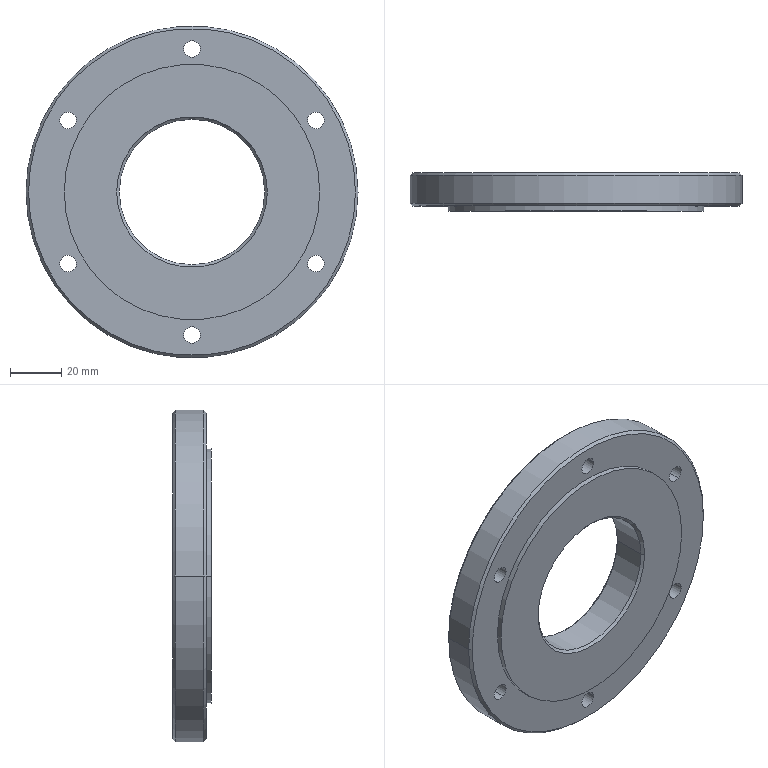Part | Creo | features CUT 7, CURVE 3, DATUM PLANE 3, CHAMFER 1, COORDINATE SYSTEM 1, PATTERN 1, PROTRUSION 1 | 1 solid | 47 faces | box 130 x 15 x 130 mm | volume 144210 mm3 | cylinder 30 | plane 9 | cone 8 | commonest cylinder face diameters 6.5 x12 11 x12 57 x2 100 x2 130 x2
STEP:
#1=CARTESIAN_POINT('',(0.,0.,0.));
#2=DIRECTION('',(0.,0.,1.));
#3=DIRECTION('',(1.,0.,0.));
#4=AXIS2_PLACEMENT_3D('',#1,#2,#3);
#5=CARTESIAN_POINT('',(50.,0.,0.));
#6=VERTEX_POINT('',#5);
#7=CARTESIAN_POINT('',(-50.,0.,0.));
#8=VERTEX_POINT('',#7);
#9=CARTESIAN_POINT('',(0.,0.,0.));
#10=DIRECTION('',(0.,-1.,0.));
#11=DIRECTION('',(1.,0.,0.));
#12=AXIS2_PLACEMENT_3D('',#9,#10,#11);
#13=CIRCLE('',#12,50.);
#14=EDGE_CURVE('',#6,#8,#13,.T.);
#15=ORIENTED_EDGE('',*,*,#14,.F.);
#16=CARTESIAN_POINT('',(0.,0.,0.));
#17=DIRECTION('',(0.,1.,0.));
#18=DIRECTION('',(1.,0.,0.));
#19=AXIS2_PLACEMENT_3D('',#16,#17,#18);
#20=CIRCLE('',#19,50.);
#21=EDGE_CURVE('',#6,#8,#20,.T.);
#22=ORIENTED_EDGE('',*,*,#21,.T.);
#23=EDGE_LOOP('',(#15,#22));
#24=FACE_OUTER_BOUND('',#23,.F.);
#25=CARTESIAN_POINT('',(-29.5,0.,0.));
#26=VERTEX_POINT('',#25);
#27=CARTESIAN_POINT('',(29.5,0.,0.));
#28=VERTEX_POINT('',#27);
#29=CARTESIAN_POINT('',(0.,0.,0.));
#30=DIRECTION('',(0.,1.,0.));
#31=DIRECTION('',(-1.,0.,0.));
#32=AXIS2_PLACEMENT_3D('',#29,#30,#31);
#33=CIRCLE('',#32,29.5);
#34=EDGE_CURVE('',#26,#28,#33,.T.);
#35=ORIENTED_EDGE('',*,*,#34,.F.);
#36=CARTESIAN_POINT('',(0.,0.,0.));
#37=DIRECTION('',(0.,1.,0.));
#38=DIRECTION('',(1.,0.,0.));
#39=AXIS2_PLACEMENT_3D('',#36,#37,#38);
#40=CIRCLE('',#39,29.5);
#41=EDGE_CURVE('',#28,#26,#40,.T.);
#42=ORIENTED_EDGE('',*,*,#41,.F.);
#43=EDGE_LOOP('',(#35,#42));
#44=FACE_BOUND('',#43,.F.);
#45=CARTESIAN_POINT('',(0.,0.,0.));
#46=DIRECTION('',(0.,1.,0.));
#47=DIRECTION('',(1.,0.,0.));
#48=AXIS2_PLACEMENT_3D('',#45,#46,#47);
#49=PLANE('',#48);
#50=ADVANCED_FACE('',(#24,#44),#49,.F.);
#51=CARTESIAN_POINT('',(50.,2.,0.));
#52=VERTEX_POINT('',#51);
#53=CARTESIAN_POINT('',(50.,0.,0.));
#54=DIRECTION('',(0.,1.,0.));
#55=VECTOR('',#54,2.);
#56=LINE('',#53,#55);
#57=EDGE_CURVE('',#6,#52,#56,.T.);
#58=ORIENTED_EDGE('',*,*,#57,.F.);
#59=ORIENTED_EDGE('',*,*,#14,.T.);
#60=CARTESIAN_POINT('',(-50.,2.,0.));
#61=VERTEX_POINT('',#60);
#62=CARTESIAN_POINT('',(-50.,0.,0.));
#63=DIRECTION('',(0.,1.,0.));
#64=VECTOR('',#63,2.);
#65=LINE('',#62,#64);
#66=EDGE_CURVE('',#8,#61,#65,.T.);
#67=ORIENTED_EDGE('',*,*,#66,.T.);
#68=CARTESIAN_POINT('',(0.,2.,0.));
#69=DIRECTION('',(0.,-1.,0.));
#70=DIRECTION('',(1.,0.,0.));
#71=AXIS2_PLACEMENT_3D('',#68,#69,#70);
#72=CIRCLE('',#71,50.);
#73=EDGE_CURVE('',#52,#61,#72,.T.);
#74=ORIENTED_EDGE('',*,*,#73,.F.);
#75=EDGE_LOOP('',(#58,#59,#67,#74));
#76=FACE_OUTER_BOUND('',#75,.F.);
#77=CARTESIAN_POINT('',(0.,0.,0.));
#78=DIRECTION('',(0.,1.,0.));
#79=DIRECTION('',(1.,0.,0.));
#80=AXIS2_PLACEMENT_3D('',#77,#78,#79);
#81=CYLINDRICAL_SURFACE('',#80,50.);
#82=ADVANCED_FACE('',(#76),#81,.T.);
#83=ORIENTED_EDGE('',*,*,#57,.T.);
#84=CARTESIAN_POINT('',(0.,2.,0.));
#85=DIRECTION('',(0.,1.,0.));
#86=DIRECTION('',(1.,0.,0.));
#87=AXIS2_PLACEMENT_3D('',#84,#85,#86);
#88=CIRCLE('',#87,50.);
#89=EDGE_CURVE('',#52,#61,#88,.T.);
#90=ORIENTED_EDGE('',*,*,#89,.T.);
#91=ORIENTED_EDGE('',*,*,#66,.F.);
#92=ORIENTED_EDGE('',*,*,#21,.F.);
#93=EDGE_LOOP('',(#83,#90,#91,#92));
#94=FACE_OUTER_BOUND('',#93,.F.);
#95=CARTESIAN_POINT('',(0.,0.,0.));
#96=DIRECTION('',(0.,1.,0.));
#97=DIRECTION('',(1.,0.,0.));
#98=AXIS2_PLACEMENT_3D('',#95,#96,#97);
#99=CYLINDRICAL_SURFACE('',#98,50.);
#100=ADVANCED_FACE('',(#94),#99,.T.);
#101=CARTESIAN_POINT('',(-64.,2.,0.));
#102=VERTEX_POINT('',#101);
#103=CARTESIAN_POINT('',(64.,2.,0.));
#104=VERTEX_POINT('',#103);
#105=CARTESIAN_POINT('',(0.,2.,0.));
#106=DIRECTION('',(0.,1.,0.));
#107=DIRECTION('',(-1.,0.,0.));
#108=AXIS2_PLACEMENT_3D('',#105,#106,#107);
#109=CIRCLE('',#108,64.);
#110=EDGE_CURVE('',#102,#104,#109,.T.);
#111=ORIENTED_EDGE('',*,*,#110,.T.);
#112=CARTESIAN_POINT('',(0.,2.,0.));
#113=DIRECTION('',(0.,1.,0.));
#114=DIRECTION('',(1.,0.,0.));
#115=AXIS2_PLACEMENT_3D('',#112,#113,#114);
#116=CIRCLE('',#115,64.);
#117=EDGE_CURVE('',#104,#102,#116,.T.);
#118=ORIENTED_EDGE('',*,*,#117,.T.);
#119=EDGE_LOOP('',(#111,#118));
#120=FACE_OUTER_BOUND('',#119,.F.);
#121=CARTESIAN_POINT('',(3.25,2.,-56.));
#122=VERTEX_POINT('',#121);
#123=CARTESIAN_POINT('',(-3.25,2.,-56.));
#124=VERTEX_POINT('',#123);
#125=CARTESIAN_POINT('',(0.,2.,-56.));
#126=DIRECTION('',(0.,1.,0.));
#127=DIRECTION('',(1.,0.,0.));
#128=AXIS2_PLACEMENT_3D('',#125,#126,#127);
#129=CIRCLE('',#128,3.25);
#130=EDGE_CURVE('',#122,#124,#129,.T.);
#131=ORIENTED_EDGE('',*,*,#130,.F.);
#132=CARTESIAN_POINT('',(0.,2.,-56.));
#133=DIRECTION('',(0.,1.,0.));
#134=DIRECTION('',(-1.,0.,0.));
#135=AXIS2_PLACEMENT_3D('',#132,#133,#134);
#136=CIRCLE('',#135,3.25);
#137=EDGE_CURVE('',#124,#122,#136,.T.);
#138=ORIENTED_EDGE('',*,*,#137,.F.);
#139=EDGE_LOOP('',(#131,#138));
#140=FACE_BOUND('',#139,.F.);
#141=CARTESIAN_POINT('',(-46.872,2.,-30.815));
#142=VERTEX_POINT('',#141);
#143=CARTESIAN_POINT('',(-50.122,2.,-25.185));
#144=VERTEX_POINT('',#143);
#145=CARTESIAN_POINT('',(-48.497,2.,-28.));
#146=DIRECTION('',(0.,1.,0.));
#147=DIRECTION('',(0.5,0.,-0.866));
#148=AXIS2_PLACEMENT_3D('',#145,#146,#147);
#149=CIRCLE('',#148,3.25);
#150=EDGE_CURVE('',#142,#144,#149,.T.);
#151=ORIENTED_EDGE('',*,*,#150,.F.);
#152=CARTESIAN_POINT('',(-48.497,2.,-28.));
#153=DIRECTION('',(0.,1.,0.));
#154=DIRECTION('',(-0.5,0.,0.866));
#155=AXIS2_PLACEMENT_3D('',#152,#153,#154);
#156=CIRCLE('',#155,3.25);
#157=EDGE_CURVE('',#144,#142,#156,.T.);
#158=ORIENTED_EDGE('',*,*,#157,.F.);
#159=EDGE_LOOP('',(#151,#158));
#160=FACE_BOUND('',#159,.F.);
#161=CARTESIAN_POINT('',(-50.122,2.,25.185));
#162=VERTEX_POINT('',#161);
#163=CARTESIAN_POINT('',(-46.872,2.,30.815));
#164=VERTEX_POINT('',#163);
#165=CARTESIAN_POINT('',(-48.497,2.,28.));
#166=DIRECTION('',(0.,1.,0.));
#167=DIRECTION('',(-0.5,0.,-0.866));
#168=AXIS2_PLACEMENT_3D('',#165,#166,#167);
#169=CIRCLE('',#168,3.25);
#170=EDGE_CURVE('',#162,#164,#169,.T.);
#171=ORIENTED_EDGE('',*,*,#170,.F.);
#172=CARTESIAN_POINT('',(-48.497,2.,28.));
#173=DIRECTION('',(0.,1.,0.));
#174=DIRECTION('',(0.5,0.,0.866));
#175=AXIS2_PLACEMENT_3D('',#172,#173,#174);
#176=CIRCLE('',#175,3.25);
#177=EDGE_CURVE('',#164,#162,#176,.T.);
#178=ORIENTED_EDGE('',*,*,#177,.F.);
#179=EDGE_LOOP('',(#171,#178));
#180=FACE_BOUND('',#179,.F.);
#181=CARTESIAN_POINT('',(-3.25,2.,56.));
#182=VERTEX_POINT('',#181);
#183=CARTESIAN_POINT('',(3.25,2.,56.));
#184=VERTEX_POINT('',#183);
#185=CARTESIAN_POINT('',(0.,2.,56.));
#186=DIRECTION('',(0.,1.,0.));
#187=DIRECTION('',(-1.,0.,0.));
#188=AXIS2_PLACEMENT_3D('',#185,#186,#187);
#189=CIRCLE('',#188,3.25);
#190=EDGE_CURVE('',#182,#184,#189,.T.);
#191=ORIENTED_EDGE('',*,*,#190,.F.);
#192=CARTESIAN_POINT('',(0.,2.,56.));
#193=DIRECTION('',(0.,1.,0.));
#194=DIRECTION('',(1.,0.,0.));
#195=AXIS2_PLACEMENT_3D('',#192,#193,#194);
#196=CIRCLE('',#195,3.25);
#197=EDGE_CURVE('',#184,#182,#196,.T.);
#198=ORIENTED_EDGE('',*,*,#197,.F.);
#199=EDGE_LOOP('',(#191,#198));
#200=FACE_BOUND('',#199,.F.);
#201=CARTESIAN_POINT('',(46.872,2.,30.815));
#202=VERTEX_POINT('',#201);
#203=CARTESIAN_POINT('',(50.122,2.,25.185));
#204=VERTEX_POINT('',#203);
#205=CARTESIAN_POINT('',(48.497,2.,28.));
#206=DIRECTION('',(0.,1.,0.));
#207=DIRECTION('',(-0.5,0.,0.866));
#208=AXIS2_PLACEMENT_3D('',#205,#206,#207);
#209=CIRCLE('',#208,3.25);
#210=EDGE_CURVE('',#202,#204,#209,.T.);
#211=ORIENTED_EDGE('',*,*,#210,.F.);
#212=CARTESIAN_POINT('',(48.497,2.,28.));
#213=DIRECTION('',(0.,1.,0.));
#214=DIRECTION('',(0.5,0.,-0.866));
#215=AXIS2_PLACEMENT_3D('',#212,#213,#214);
#216=CIRCLE('',#215,3.25);
#217=EDGE_CURVE('',#204,#202,#216,.T.);
#218=ORIENTED_EDGE('',*,*,#217,.F.);
#219=EDGE_LOOP('',(#211,#218));
#220=FACE_BOUND('',#219,.F.);
#221=CARTESIAN_POINT('',(50.122,2.,-25.185));
#222=VERTEX_POINT('',#221);
#223=CARTESIAN_POINT('',(46.872,2.,-30.815));
#224=VERTEX_POINT('',#223);
#225=CARTESIAN_POINT('',(48.497,2.,-28.));
#226=DIRECTION('',(0.,1.,0.));
#227=DIRECTION('',(0.5,0.,0.866));
#228=AXIS2_PLACEMENT_3D('',#225,#226,#227);
#229=CIRCLE('',#228,3.25);
#230=EDGE_CURVE('',#222,#224,#229,.T.);
#231=ORIENTED_EDGE('',*,*,#230,.F.);
#232=CARTESIAN_POINT('',(48.497,2.,-28.));
#233=DIRECTION('',(0.,1.,0.));
#234=DIRECTION('',(-0.5,0.,-0.866));
#235=AXIS2_PLACEMENT_3D('',#232,#233,#234);
#236=CIRCLE('',#235,3.25);
#237=EDGE_CURVE('',#224,#222,#236,.T.);
#238=ORIENTED_EDGE('',*,*,#237,.F.);
#239=EDGE_LOOP('',(#231,#238));
#240=FACE_BOUND('',#239,.F.);
#241=ORIENTED_EDGE('',*,*,#89,.F.);
#242=ORIENTED_EDGE('',*,*,#73,.T.);
#243=EDGE_LOOP('',(#241,#242));
#244=FACE_BOUND('',#243,.F.);
#245=CARTESIAN_POINT('',(0.,2.,0.));
#246=DIRECTION('',(0.,1.,0.));
#247=DIRECTION('',(1.,0.,0.));
#248=AXIS2_PLACEMENT_3D('',#245,#246,#247);
#249=PLANE('',#248);
#250=ADVANCED_FACE('',(#120,#140,#160,#180,#200,#220,#240,#244),#249,.F.);
#251=CARTESIAN_POINT('',(3.25,8.,-56.));
#252=VERTEX_POINT('',#251);
#253=CARTESIAN_POINT('',(-3.25,8.,-56.));
#254=VERTEX_POINT('',#253);
#255=CARTESIAN_POINT('',(0.,8.,-56.));
#256=DIRECTION('',(0.,1.,0.));
#257=DIRECTION('',(1.,0.,0.));
#258=AXIS2_PLACEMENT_3D('',#255,#256,#257);
#259=CIRCLE('',#258,3.25);
#260=EDGE_CURVE('',#252,#254,#259,.T.);
#261=ORIENTED_EDGE('',*,*,#260,.F.);
#262=CARTESIAN_POINT('',(3.25,8.,-56.));
#263=DIRECTION('',(0.,-1.,0.));
#264=VECTOR('',#263,6.);
#265=LINE('',#262,#264);
#266=EDGE_CURVE('',#252,#122,#265,.T.);
#267=ORIENTED_EDGE('',*,*,#266,.T.);
#268=ORIENTED_EDGE('',*,*,#130,.T.);
#269=CARTESIAN_POINT('',(-3.25,8.,-56.));
#270=DIRECTION('',(0.,-1.,0.));
#271=VECTOR('',#270,6.);
#272=LINE('',#269,#271);
#273=EDGE_CURVE('',#254,#124,#272,.T.);
#274=ORIENTED_EDGE('',*,*,#273,.F.);
#275=EDGE_LOOP('',(#261,#267,#268,#274));
#276=FACE_OUTER_BOUND('',#275,.F.);
#277=CARTESIAN_POINT('',(0.,15.,-56.));
#278=DIRECTION('',(0.,1.,0.));
#279=DIRECTION('',(1.,0.,0.));
#280=AXIS2_PLACEMENT_3D('',#277,#278,#279);
#281=CYLINDRICAL_SURFACE('',#280,3.25);
#282=ADVANCED_FACE('',(#276),#281,.F.);
#283=CARTESIAN_POINT('',(5.5,8.,-56.));
#284=VERTEX_POINT('',#283);
#285=CARTESIAN_POINT('',(-5.5,8.,-56.));
#286=VERTEX_POINT('',#285);
#287=CARTESIAN_POINT('',(0.,8.,-56.));
#288=DIRECTION('',(0.,1.,0.));
#289=DIRECTION('',(1.,0.,0.));
#290=AXIS2_PLACEMENT_3D('',#287,#288,#289);
#291=CIRCLE('',#290,5.5);
#292=EDGE_CURVE('',#284,#286,#291,.T.);
#293=ORIENTED_EDGE('',*,*,#292,.F.);
#294=CARTESIAN_POINT('',(0.,8.,-56.));
#295=DIRECTION('',(0.,1.,0.));
#296=DIRECTION('',(-1.,0.,0.));
#297=AXIS2_PLACEMENT_3D('',#294,#295,#296);
#298=CIRCLE('',#297,5.5);
#299=EDGE_CURVE('',#286,#284,#298,.T.);
#300=ORIENTED_EDGE('',*,*,#299,.F.);
#301=EDGE_LOOP('',(#293,#300));
#302=FACE_OUTER_BOUND('',#301,.F.);
#303=ORIENTED_EDGE('',*,*,#260,.T.);
#304=CARTESIAN_POINT('',(0.,8.,-56.));
#305=DIRECTION('',(0.,1.,0.));
#306=DIRECTION('',(-1.,0.,0.));
#307=AXIS2_PLACEMENT_3D('',#304,#305,#306);
#308=CIRCLE('',#307,3.25);
#309=EDGE_CURVE('',#254,#252,#308,.T.);
#310=ORIENTED_EDGE('',*,*,#309,.T.);
#311=EDGE_LOOP('',(#303,#310));
#312=FACE_BOUND('',#311,.F.);
#313=CARTESIAN_POINT('',(0.,8.,0.));
#314=DIRECTION('',(0.,1.,0.));
#315=DIRECTION('',(1.,0.,0.));
#316=AXIS2_PLACEMENT_3D('',#313,#314,#315);
#317=PLANE('',#316);
#318=ADVANCED_FACE('',(#302,#312),#317,.T.);
#319=CARTESIAN_POINT('',(53.997,8.,-28.));
#320=VERTEX_POINT('',#319);
#321=CARTESIAN_POINT('',(42.997,8.,-28.));
#322=VERTEX_POINT('',#321);
#323=CARTESIAN_POINT('',(48.497,8.,-28.));
#324=DIRECTION('',(0.,1.,0.));
#325=DIRECTION('',(1.,0.,0.));
#326=AXIS2_PLACEMENT_3D('',#323,#324,#325);
#327=CIRCLE('',#326,5.5);
#328=EDGE_CURVE('',#320,#322,#327,.T.);
#329=ORIENTED_EDGE('',*,*,#328,.F.);
#330=CARTESIAN_POINT('',(48.497,8.,-28.));
#331=DIRECTION('',(0.,1.,0.));
#332=DIRECTION('',(-1.,0.,0.));
#333=AXIS2_PLACEMENT_3D('',#330,#331,#332);
#334=CIRCLE('',#333,5.5);
#335=EDGE_CURVE('',#322,#320,#334,.T.);
#336=ORIENTED_EDGE('',*,*,#335,.F.);
#337=EDGE_LOOP('',(#329,#336));
#338=FACE_OUTER_BOUND('',#337,.F.);
#339=CARTESIAN_POINT('',(50.122,8.,-25.185));
#340=VERTEX_POINT('',#339);
#341=CARTESIAN_POINT('',(46.872,8.,-30.815));
#342=VERTEX_POINT('',#341);
#343=CARTESIAN_POINT('',(48.497,8.,-28.));
#344=DIRECTION('',(0.,1.,0.));
#345=DIRECTION('',(0.5,0.,0.866));
#346=AXIS2_PLACEMENT_3D('',#343,#344,#345);
#347=CIRCLE('',#346,3.25);
#348=EDGE_CURVE('',#340,#342,#347,.T.);
#349=ORIENTED_EDGE('',*,*,#348,.T.);
#350=CARTESIAN_POINT('',(48.497,8.,-28.));
#351=DIRECTION('',(0.,1.,0.));
#352=DIRECTION('',(-0.5,0.,-0.866));
#353=AXIS2_PLACEMENT_3D('',#350,#351,#352);
#354=CIRCLE('',#353,3.25);
#355=EDGE_CURVE('',#342,#340,#354,.T.);
#356=ORIENTED_EDGE('',*,*,#355,.T.);
#357=EDGE_LOOP('',(#349,#356));
#358=FACE_BOUND('',#357,.F.);
#359=CARTESIAN_POINT('',(0.,8.,0.));
#360=DIRECTION('',(0.,1.,0.));
#361=DIRECTION('',(1.,0.,0.));
#362=AXIS2_PLACEMENT_3D('',#359,#360,#361);
#363=PLANE('',#362);
#364=ADVANCED_FACE('',(#338,#358),#363,.T.);
#365=CARTESIAN_POINT('',(53.997,8.,28.));
#366=VERTEX_POINT('',#365);
#367=CARTESIAN_POINT('',(42.997,8.,28.));
#368=VERTEX_POINT('',#367);
#369=CARTESIAN_POINT('',(48.497,8.,28.));
#370=DIRECTION('',(0.,1.,0.));
#371=DIRECTION('',(1.,0.,0.));
#372=AXIS2_PLACEMENT_3D('',#369,#370,#371);
#373=CIRCLE('',#372,5.5);
#374=EDGE_CURVE('',#366,#368,#373,.T.);
#375=ORIENTED_EDGE('',*,*,#374,.F.);
#376=CARTESIAN_POINT('',(48.497,8.,28.));
#377=DIRECTION('',(0.,1.,0.));
#378=DIRECTION('',(-1.,0.,0.));
#379=AXIS2_PLACEMENT_3D('',#376,#377,#378);
#380=CIRCLE('',#379,5.5);
#381=EDGE_CURVE('',#368,#366,#380,.T.);
#382=ORIENTED_EDGE('',*,*,#381,.F.);
#383=EDGE_LOOP('',(#375,#382));
#384=FACE_OUTER_BOUND('',#383,.F.);
#385=CARTESIAN_POINT('',(46.872,8.,30.815));
#386=VERTEX_POINT('',#385);
#387=CARTESIAN_POINT('',(50.122,8.,25.185));
#388=VERTEX_POINT('',#387);
#389=CARTESIAN_POINT('',(48.497,8.,28.));
#390=DIRECTION('',(0.,1.,0.));
#391=DIRECTION('',(-0.5,0.,0.866));
#392=AXIS2_PLACEMENT_3D('',#389,#390,#391);
#393=CIRCLE('',#392,3.25);
#394=EDGE_CURVE('',#386,#388,#393,.T.);
#395=ORIENTED_EDGE('',*,*,#394,.T.);
#396=CARTESIAN_POINT('',(48.497,8.,28.));
#397=DIRECTION('',(0.,1.,0.));
#398=DIRECTION('',(0.5,0.,-0.866));
#399=AXIS2_PLACEMENT_3D('',#396,#397,#398);
#400=CIRCLE('',#399,3.25);
#401=EDGE_CURVE('',#388,#386,#400,.T.);
#402=ORIENTED_EDGE('',*,*,#401,.T.);
#403=EDGE_LOOP('',(#395,#402));
#404=FACE_BOUND('',#403,.F.);
#405=CARTESIAN_POINT('',(0.,8.,0.));
#406=DIRECTION('',(0.,1.,0.));
#407=DIRECTION('',(1.,0.,0.));
#408=AXIS2_PLACEMENT_3D('',#405,#406,#407);
#409=PLANE('',#408);
#410=ADVANCED_FACE('',(#384,#404),#409,.T.);
#411=CARTESIAN_POINT('',(5.5,8.,56.));
#412=VERTEX_POINT('',#411);
#413=CARTESIAN_POINT('',(-5.5,8.,56.));
#414=VERTEX_POINT('',#413);
#415=CARTESIAN_POINT('',(0.,8.,56.));
#416=DIRECTION('',(0.,1.,0.));
#417=DIRECTION('',(1.,0.,0.));
#418=AXIS2_PLACEMENT_3D('',#415,#416,#417);
#419=CIRCLE('',#418,5.5);
#420=EDGE_CURVE('',#412,#414,#419,.T.);
#421=ORIENTED_EDGE('',*,*,#420,.F.);
#422=CARTESIAN_POINT('',(0.,8.,56.));
#423=DIRECTION('',(0.,1.,0.));
#424=DIRECTION('',(-1.,0.,0.));
#425=AXIS2_PLACEMENT_3D('',#422,#423,#424);
#426=CIRCLE('',#425,5.5);
#427=EDGE_CURVE('',#414,#412,#426,.T.);
#428=ORIENTED_EDGE('',*,*,#427,.F.);
#429=EDGE_LOOP('',(#421,#428));
#430=FACE_OUTER_BOUND('',#429,.F.);
#431=CARTESIAN_POINT('',(-3.25,8.,56.));
#432=VERTEX_POINT('',#431);
#433=CARTESIAN_POINT('',(3.25,8.,56.));
#434=VERTEX_POINT('',#433);
#435=CARTESIAN_POINT('',(0.,8.,56.));
#436=DIRECTION('',(0.,1.,0.));
#437=DIRECTION('',(-1.,0.,0.));
#438=AXIS2_PLACEMENT_3D('',#435,#436,#437);
#439=CIRCLE('',#438,3.25);
#440=EDGE_CURVE('',#432,#434,#439,.T.);
#441=ORIENTED_EDGE('',*,*,#440,.T.);
#442=CARTESIAN_POINT('',(0.,8.,56.));
#443=DIRECTION('',(0.,1.,0.));
#444=DIRECTION('',(1.,0.,0.));
#445=AXIS2_PLACEMENT_3D('',#442,#443,#444);
#446=CIRCLE('',#445,3.25);
#447=EDGE_CURVE('',#434,#432,#446,.T.);
#448=ORIENTED_EDGE('',*,*,#447,.T.);
#449=EDGE_LOOP('',(#441,#448));
#450=FACE_BOUND('',#449,.F.);
#451=CARTESIAN_POINT('',(0.,8.,0.));
#452=DIRECTION('',(0.,1.,0.));
#453=DIRECTION('',(1.,0.,0.));
#454=AXIS2_PLACEMENT_3D('',#451,#452,#453);
#455=PLANE('',#454);
#456=ADVANCED_FACE('',(#430,#450),#455,.T.);
#457=CARTESIAN_POINT('',(-42.997,8.,28.));
#458=VERTEX_POINT('',#457);
#459=CARTESIAN_POINT('',(-53.997,8.,28.));
#460=VERTEX_POINT('',#459);
#461=CARTESIAN_POINT('',(-48.497,8.,28.));
#462=DIRECTION('',(0.,1.,0.));
#463=DIRECTION('',(1.,0.,0.));
#464=AXIS2_PLACEMENT_3D('',#461,#462,#463);
#465=CIRCLE('',#464,5.5);
#466=EDGE_CURVE('',#458,#460,#465,.T.);
#467=ORIENTED_EDGE('',*,*,#466,.F.);
#468=CARTESIAN_POINT('',(-48.497,8.,28.));
#469=DIRECTION('',(0.,1.,0.));
#470=DIRECTION('',(-1.,0.,0.));
#471=AXIS2_PLACEMENT_3D('',#468,#469,#470);
#472=CIRCLE('',#471,5.5);
#473=EDGE_CURVE('',#460,#458,#472,.T.);
#474=ORIENTED_EDGE('',*,*,#473,.F.);
#475=EDGE_LOOP('',(#467,#474));
#476=FACE_OUTER_BOUND('',#475,.F.);
#477=CARTESIAN_POINT('',(-50.122,8.,25.185));
#478=VERTEX_POINT('',#477);
#479=CARTESIAN_POINT('',(-46.872,8.,30.815));
#480=VERTEX_POINT('',#479);
#481=CARTESIAN_POINT('',(-48.497,8.,28.));
#482=DIRECTION('',(0.,1.,0.));
#483=DIRECTION('',(-0.5,0.,-0.866));
#484=AXIS2_PLACEMENT_3D('',#481,#482,#483);
#485=CIRCLE('',#484,3.25);
#486=EDGE_CURVE('',#478,#480,#485,.T.);
#487=ORIENTED_EDGE('',*,*,#486,.T.);
#488=CARTESIAN_POINT('',(-48.497,8.,28.));
#489=DIRECTION('',(0.,1.,0.));
#490=DIRECTION('',(0.5,0.,0.866));
#491=AXIS2_PLACEMENT_3D('',#488,#489,#490);
#492=CIRCLE('',#491,3.25);
#493=EDGE_CURVE('',#480,#478,#492,.T.);
#494=ORIENTED_EDGE('',*,*,#493,.T.);
#495=EDGE_LOOP('',(#487,#494));
#496=FACE_BOUND('',#495,.F.);
#497=CARTESIAN_POINT('',(0.,8.,0.));
#498=DIRECTION('',(0.,1.,0.));
#499=DIRECTION('',(1.,0.,0.));
#500=AXIS2_PLACEMENT_3D('',#497,#498,#499);
#501=PLANE('',#500);
#502=ADVANCED_FACE('',(#476,#496),#501,.T.);
#503=CARTESIAN_POINT('',(-42.997,8.,-28.));
#504=VERTEX_POINT('',#503);
#505=CARTESIAN_POINT('',(-53.997,8.,-28.));
#506=VERTEX_POINT('',#505);
#507=CARTESIAN_POINT('',(-48.497,8.,-28.));
#508=DIRECTION('',(0.,1.,0.));
#509=DIRECTION('',(1.,0.,0.));
#510=AXIS2_PLACEMENT_3D('',#507,#508,#509);
#511=CIRCLE('',#510,5.5);
#512=EDGE_CURVE('',#504,#506,#511,.T.);
#513=ORIENTED_EDGE('',*,*,#512,.F.);
#514=CARTESIAN_POINT('',(-48.497,8.,-28.));
#515=DIRECTION('',(0.,1.,0.));
#516=DIRECTION('',(-1.,0.,0.));
#517=AXIS2_PLACEMENT_3D('',#514,#515,#516);
#518=CIRCLE('',#517,5.5);
#519=EDGE_CURVE('',#506,#504,#518,.T.);
#520=ORIENTED_EDGE('',*,*,#519,.F.);
#521=EDGE_LOOP('',(#513,#520));
#522=FACE_OUTER_BOUND('',#521,.F.);
#523=CARTESIAN_POINT('',(-46.872,8.,-30.815));
#524=VERTEX_POINT('',#523);
#525=CARTESIAN_POINT('',(-50.122,8.,-25.185));
#526=VERTEX_POINT('',#525);
#527=CARTESIAN_POINT('',(-48.497,8.,-28.));
#528=DIRECTION('',(0.,1.,0.));
#529=DIRECTION('',(0.5,0.,-0.866));
#530=AXIS2_PLACEMENT_3D('',#527,#528,#529);
#531=CIRCLE('',#530,3.25);
#532=EDGE_CURVE('',#524,#526,#531,.T.);
#533=ORIENTED_EDGE('',*,*,#532,.T.);
#534=CARTESIAN_POINT('',(-48.497,8.,-28.));
#535=DIRECTION('',(0.,1.,0.));
#536=DIRECTION('',(-0.5,0.,0.866));
#537=AXIS2_PLACEMENT_3D('',#534,#535,#536);
#538=CIRCLE('',#537,3.25);
#539=EDGE_CURVE('',#526,#524,#538,.T.);
#540=ORIENTED_EDGE('',*,*,#539,.T.);
#541=EDGE_LOOP('',(#533,#540));
#542=FACE_BOUND('',#541,.F.);
#543=CARTESIAN_POINT('',(0.,8.,0.));
#544=DIRECTION('',(0.,1.,0.));
#545=DIRECTION('',(1.,0.,0.));
#546=AXIS2_PLACEMENT_3D('',#543,#544,#545);
#547=PLANE('',#546);
#548=ADVANCED_FACE('',(#522,#542),#547,.T.);
#549=CARTESIAN_POINT('',(5.5,15.,-56.));
#550=VERTEX_POINT('',#549);
#551=CARTESIAN_POINT('',(-5.5,15.,-56.));
#552=VERTEX_POINT('',#551);
#553=CARTESIAN_POINT('',(0.,15.,-56.));
#554=DIRECTION('',(0.,1.,0.));
#555=DIRECTION('',(1.,0.,0.));
#556=AXIS2_PLACEMENT_3D('',#553,#554,#555);
#557=CIRCLE('',#556,5.5);
#558=EDGE_CURVE('',#550,#552,#557,.T.);
#559=ORIENTED_EDGE('',*,*,#558,.F.);
#560=CARTESIAN_POINT('',(5.5,15.,-56.));
#561=DIRECTION('',(0.,-1.,0.));
#562=VECTOR('',#561,7.);
#563=LINE('',#560,#562);
#564=EDGE_CURVE('',#550,#284,#563,.T.);
#565=ORIENTED_EDGE('',*,*,#564,.T.);
#566=ORIENTED_EDGE('',*,*,#292,.T.);
#567=CARTESIAN_POINT('',(-5.5,15.,-56.));
#568=DIRECTION('',(0.,-1.,0.));
#569=VECTOR('',#568,7.);
#570=LINE('',#567,#569);
#571=EDGE_CURVE('',#552,#286,#570,.T.);
#572=ORIENTED_EDGE('',*,*,#571,.F.);
#573=EDGE_LOOP('',(#559,#565,#566,#572));
#574=FACE_OUTER_BOUND('',#573,.F.);
#575=CARTESIAN_POINT('',(0.,15.,-56.));
#576=DIRECTION('',(0.,1.,0.));
#577=DIRECTION('',(1.,0.,0.));
#578=AXIS2_PLACEMENT_3D('',#575,#576,#577);
#579=CYLINDRICAL_SURFACE('',#578,5.5);
#580=ADVANCED_FACE('',(#574),#579,.F.);
#581=CARTESIAN_POINT('',(-64.,15.,0.));
#582=VERTEX_POINT('',#581);
#583=CARTESIAN_POINT('',(64.,15.,0.));
#584=VERTEX_POINT('',#583);
#585=CARTESIAN_POINT('',(0.,15.,0.));
#586=DIRECTION('',(0.,1.,0.));
#587=DIRECTION('',(-1.,0.,0.));
#588=AXIS2_PLACEMENT_3D('',#585,#586,#587);
#589=CIRCLE('',#588,64.);
#590=EDGE_CURVE('',#582,#584,#589,.T.);
#591=ORIENTED_EDGE('',*,*,#590,.F.);
#592=CARTESIAN_POINT('',(0.,15.,0.));
#593=DIRECTION('',(0.,1.,0.));
#594=DIRECTION('',(1.,0.,0.));
#595=AXIS2_PLACEMENT_3D('',#592,#593,#594);
#596=CIRCLE('',#595,64.);
#597=EDGE_CURVE('',#584,#582,#596,.T.);
#598=ORIENTED_EDGE('',*,*,#597,.F.);
#599=EDGE_LOOP('',(#591,#598));
#600=FACE_OUTER_BOUND('',#599,.F.);
#601=CARTESIAN_POINT('',(53.997,15.,-28.));
#602=VERTEX_POINT('',#601);
#603=CARTESIAN_POINT('',(42.997,15.,-28.));
#604=VERTEX_POINT('',#603);
#605=CARTESIAN_POINT('',(48.497,15.,-28.));
#606=DIRECTION('',(0.,1.,0.));
#607=DIRECTION('',(1.,0.,0.));
#608=AXIS2_PLACEMENT_3D('',#605,#606,#607);
#609=CIRCLE('',#608,5.5);
#610=EDGE_CURVE('',#602,#604,#609,.T.);
#611=ORIENTED_EDGE('',*,*,#610,.T.);
#612=CARTESIAN_POINT('',(48.497,15.,-28.));
#613=DIRECTION('',(0.,1.,0.));
#614=DIRECTION('',(-1.,0.,0.));
#615=AXIS2_PLACEMENT_3D('',#612,#613,#614);
#616=CIRCLE('',#615,5.5);
#617=EDGE_CURVE('',#604,#602,#616,.T.);
#618=ORIENTED_EDGE('',*,*,#617,.T.);
#619=EDGE_LOOP('',(#611,#618));
#620=FACE_BOUND('',#619,.F.);
#621=CARTESIAN_POINT('',(53.997,15.,28.));
#622=VERTEX_POINT('',#621);
#623=CARTESIAN_POINT('',(42.997,15.,28.));
#624=VERTEX_POINT('',#623);
#625=CARTESIAN_POINT('',(48.497,15.,28.));
#626=DIRECTION('',(0.,1.,0.));
#627=DIRECTION('',(1.,0.,0.));
#628=AXIS2_PLACEMENT_3D('',#625,#626,#627);
#629=CIRCLE('',#628,5.5);
#630=EDGE_CURVE('',#622,#624,#629,.T.);
#631=ORIENTED_EDGE('',*,*,#630,.T.);
#632=CARTESIAN_POINT('',(48.497,15.,28.));
#633=DIRECTION('',(0.,1.,0.));
#634=DIRECTION('',(-1.,0.,0.));
#635=AXIS2_PLACEMENT_3D('',#632,#633,#634);
#636=CIRCLE('',#635,5.5);
#637=EDGE_CURVE('',#624,#622,#636,.T.);
#638=ORIENTED_EDGE('',*,*,#637,.T.);
#639=EDGE_LOOP('',(#631,#638));
#640=FACE_BOUND('',#639,.F.);
#641=CARTESIAN_POINT('',(5.5,15.,56.));
#642=VERTEX_POINT('',#641);
#643=CARTESIAN_POINT('',(-5.5,15.,56.));
#644=VERTEX_POINT('',#643);
#645=CARTESIAN_POINT('',(0.,15.,56.));
#646=DIRECTION('',(0.,1.,0.));
#647=DIRECTION('',(1.,0.,0.));
#648=AXIS2_PLACEMENT_3D('',#645,#646,#647);
#649=CIRCLE('',#648,5.5);
#650=EDGE_CURVE('',#642,#644,#649,.T.);
#651=ORIENTED_EDGE('',*,*,#650,.T.);
#652=CARTESIAN_POINT('',(0.,15.,56.));
#653=DIRECTION('',(0.,1.,0.));
#654=DIRECTION('',(-1.,0.,0.));
#655=AXIS2_PLACEMENT_3D('',#652,#653,#654);
#656=CIRCLE('',#655,5.5);
#657=EDGE_CURVE('',#644,#642,#656,.T.);
#658=ORIENTED_EDGE('',*,*,#657,.T.);
#659=EDGE_LOOP('',(#651,#658));
#660=FACE_BOUND('',#659,.F.);
#661=CARTESIAN_POINT('',(-42.997,15.,28.));
#662=VERTEX_POINT('',#661);
#663=CARTESIAN_POINT('',(-53.997,15.,28.));
#664=VERTEX_POINT('',#663);
#665=CARTESIAN_POINT('',(-48.497,15.,28.));
#666=DIRECTION('',(0.,1.,0.));
#667=DIRECTION('',(1.,0.,0.));
#668=AXIS2_PLACEMENT_3D('',#665,#666,#667);
#669=CIRCLE('',#668,5.5);
#670=EDGE_CURVE('',#662,#664,#669,.T.);
#671=ORIENTED_EDGE('',*,*,#670,.T.);
#672=CARTESIAN_POINT('',(-48.497,15.,28.));
#673=DIRECTION('',(0.,1.,0.));
#674=DIRECTION('',(-1.,0.,0.));
#675=AXIS2_PLACEMENT_3D('',#672,#673,#674);
#676=CIRCLE('',#675,5.5);
#677=EDGE_CURVE('',#664,#662,#676,.T.);
#678=ORIENTED_EDGE('',*,*,#677,.T.);
#679=EDGE_LOOP('',(#671,#678));
#680=FACE_BOUND('',#679,.F.);
#681=CARTESIAN_POINT('',(-42.997,15.,-28.));
#682=VERTEX_POINT('',#681);
#683=CARTESIAN_POINT('',(-53.997,15.,-28.));
#684=VERTEX_POINT('',#683);
#685=CARTESIAN_POINT('',(-48.497,15.,-28.));
#686=DIRECTION('',(0.,1.,0.));
#687=DIRECTION('',(1.,0.,0.));
#688=AXIS2_PLACEMENT_3D('',#685,#686,#687);
#689=CIRCLE('',#688,5.5);
#690=EDGE_CURVE('',#682,#684,#689,.T.);
#691=ORIENTED_EDGE('',*,*,#690,.T.);
#692=CARTESIAN_POINT('',(-48.497,15.,-28.));
#693=DIRECTION('',(0.,1.,0.));
#694=DIRECTION('',(-1.,0.,0.));
#695=AXIS2_PLACEMENT_3D('',#692,#693,#694);
#696=CIRCLE('',#695,5.5);
#697=EDGE_CURVE('',#684,#682,#696,.T.);
#698=ORIENTED_EDGE('',*,*,#697,.T.);
#699=EDGE_LOOP('',(#691,#698));
#700=FACE_BOUND('',#699,.F.);
#701=ORIENTED_EDGE('',*,*,#558,.T.);
#702=CARTESIAN_POINT('',(0.,15.,-56.));
#703=DIRECTION('',(0.,1.,0.));
#704=DIRECTION('',(-1.,0.,0.));
#705=AXIS2_PLACEMENT_3D('',#702,#703,#704);
#706=CIRCLE('',#705,5.5);
#707=EDGE_CURVE('',#552,#550,#706,.T.);
#708=ORIENTED_EDGE('',*,*,#707,.T.);
#709=EDGE_LOOP('',(#701,#708));
#710=FACE_BOUND('',#709,.F.);
#711=CARTESIAN_POINT('',(-29.5,15.,0.));
#712=VERTEX_POINT('',#711);
#713=CARTESIAN_POINT('',(29.5,15.,0.));
#714=VERTEX_POINT('',#713);
#715=CARTESIAN_POINT('',(0.,15.,0.));
#716=DIRECTION('',(0.,1.,0.));
#717=DIRECTION('',(-1.,0.,0.));
#718=AXIS2_PLACEMENT_3D('',#715,#716,#717);
#719=CIRCLE('',#718,29.5);
#720=EDGE_CURVE('',#712,#714,#719,.T.);
#721=ORIENTED_EDGE('',*,*,#720,.T.);
#722=CARTESIAN_POINT('',(0.,15.,0.));
#723=DIRECTION('',(0.,1.,0.));
#724=DIRECTION('',(1.,0.,0.));
#725=AXIS2_PLACEMENT_3D('',#722,#723,#724);
#726=CIRCLE('',#725,29.5);
#727=EDGE_CURVE('',#714,#712,#726,.T.);
#728=ORIENTED_EDGE('',*,*,#727,.T.);
#729=EDGE_LOOP('',(#721,#728));
#730=FACE_BOUND('',#729,.F.);
#731=CARTESIAN_POINT('',(0.,15.,0.));
#732=DIRECTION('',(0.,1.,0.));
#733=DIRECTION('',(1.,0.,0.));
#734=AXIS2_PLACEMENT_3D('',#731,#732,#733);
#735=PLANE('',#734);
#736=ADVANCED_FACE('',(#600,#620,#640,#660,#680,#700,#710,#730),#735,.T.);
#737=ORIENTED_EDGE('',*,*,#707,.F.);
#738=ORIENTED_EDGE('',*,*,#571,.T.);
#739=ORIENTED_EDGE('',*,*,#299,.T.);
#740=ORIENTED_EDGE('',*,*,#564,.F.);
#741=EDGE_LOOP('',(#737,#738,#739,#740));
#742=FACE_OUTER_BOUND('',#741,.F.);
#743=CARTESIAN_POINT('',(0.,15.,-56.));
#744=DIRECTION('',(0.,1.,0.));
#745=DIRECTION('',(1.,0.,0.));
#746=AXIS2_PLACEMENT_3D('',#743,#744,#745);
#747=CYLINDRICAL_SURFACE('',#746,5.5);
#748=ADVANCED_FACE('',(#742),#747,.F.);
#749=ORIENTED_EDGE('',*,*,#610,.F.);
#750=CARTESIAN_POINT('',(53.997,15.,-28.));
#751=DIRECTION('',(0.,-1.,0.));
#752=VECTOR('',#751,7.);
#753=LINE('',#750,#752);
#754=EDGE_CURVE('',#602,#320,#753,.T.);
#755=ORIENTED_EDGE('',*,*,#754,.T.);
#756=ORIENTED_EDGE('',*,*,#328,.T.);
#757=CARTESIAN_POINT('',(42.997,15.,-28.));
#758=DIRECTION('',(0.,-1.,0.));
#759=VECTOR('',#758,7.);
#760=LINE('',#757,#759);
#761=EDGE_CURVE('',#604,#322,#760,.T.);
#762=ORIENTED_EDGE('',*,*,#761,.F.);
#763=EDGE_LOOP('',(#749,#755,#756,#762));
#764=FACE_OUTER_BOUND('',#763,.F.);
#765=CARTESIAN_POINT('',(48.497,15.,-28.));
#766=DIRECTION('',(0.,1.,0.));
#767=DIRECTION('',(1.,0.,0.));
#768=AXIS2_PLACEMENT_3D('',#765,#766,#767);
#769=CYLINDRICAL_SURFACE('',#768,5.5);
#770=ADVANCED_FACE('',(#764),#769,.F.);
#771=ORIENTED_EDGE('',*,*,#617,.F.);
#772=ORIENTED_EDGE('',*,*,#761,.T.);
#773=ORIENTED_EDGE('',*,*,#335,.T.);
#774=ORIENTED_EDGE('',*,*,#754,.F.);
#775=EDGE_LOOP('',(#771,#772,#773,#774));
#776=FACE_OUTER_BOUND('',#775,.F.);
#777=CARTESIAN_POINT('',(48.497,15.,-28.));
#778=DIRECTION('',(0.,1.,0.));
#779=DIRECTION('',(1.,0.,0.));
#780=AXIS2_PLACEMENT_3D('',#777,#778,#779);
#781=CYLINDRICAL_SURFACE('',#780,5.5);
#782=ADVANCED_FACE('',(#776),#781,.F.);
#783=ORIENTED_EDGE('',*,*,#630,.F.);
#784=CARTESIAN_POINT('',(53.997,15.,28.));
#785=DIRECTION('',(0.,-1.,0.));
#786=VECTOR('',#785,7.);
#787=LINE('',#784,#786);
#788=EDGE_CURVE('',#622,#366,#787,.T.);
#789=ORIENTED_EDGE('',*,*,#788,.T.);
#790=ORIENTED_EDGE('',*,*,#374,.T.);
#791=CARTESIAN_POINT('',(42.997,15.,28.));
#792=DIRECTION('',(0.,-1.,0.));
#793=VECTOR('',#792,7.);
#794=LINE('',#791,#793);
#795=EDGE_CURVE('',#624,#368,#794,.T.);
#796=ORIENTED_EDGE('',*,*,#795,.F.);
#797=EDGE_LOOP('',(#783,#789,#790,#796));
#798=FACE_OUTER_BOUND('',#797,.F.);
#799=CARTESIAN_POINT('',(48.497,15.,28.));
#800=DIRECTION('',(0.,1.,0.));
#801=DIRECTION('',(1.,0.,0.));
#802=AXIS2_PLACEMENT_3D('',#799,#800,#801);
#803=CYLINDRICAL_SURFACE('',#802,5.5);
#804=ADVANCED_FACE('',(#798),#803,.F.);
#805=ORIENTED_EDGE('',*,*,#637,.F.);
#806=ORIENTED_EDGE('',*,*,#795,.T.);
#807=ORIENTED_EDGE('',*,*,#381,.T.);
#808=ORIENTED_EDGE('',*,*,#788,.F.);
#809=EDGE_LOOP('',(#805,#806,#807,#808));
#810=FACE_OUTER_BOUND('',#809,.F.);
#811=CARTESIAN_POINT('',(48.497,15.,28.));
#812=DIRECTION('',(0.,1.,0.));
#813=DIRECTION('',(1.,0.,0.));
#814=AXIS2_PLACEMENT_3D('',#811,#812,#813);
#815=CYLINDRICAL_SURFACE('',#814,5.5);
#816=ADVANCED_FACE('',(#810),#815,.F.);
#817=ORIENTED_EDGE('',*,*,#650,.F.);
#818=CARTESIAN_POINT('',(5.5,15.,56.));
#819=DIRECTION('',(0.,-1.,0.));
#820=VECTOR('',#819,7.);
#821=LINE('',#818,#820);
#822=EDGE_CURVE('',#642,#412,#821,.T.);
#823=ORIENTED_EDGE('',*,*,#822,.T.);
#824=ORIENTED_EDGE('',*,*,#420,.T.);
#825=CARTESIAN_POINT('',(-5.5,15.,56.));
#826=DIRECTION('',(0.,-1.,0.));
#827=VECTOR('',#826,7.);
#828=LINE('',#825,#827);
#829=EDGE_CURVE('',#644,#414,#828,.T.);
#830=ORIENTED_EDGE('',*,*,#829,.F.);
#831=EDGE_LOOP('',(#817,#823,#824,#830));
#832=FACE_OUTER_BOUND('',#831,.F.);
#833=CARTESIAN_POINT('',(0.,15.,56.));
#834=DIRECTION('',(0.,1.,0.));
#835=DIRECTION('',(1.,0.,0.));
#836=AXIS2_PLACEMENT_3D('',#833,#834,#835);
#837=CYLINDRICAL_SURFACE('',#836,5.5);
#838=ADVANCED_FACE('',(#832),#837,.F.);
#839=ORIENTED_EDGE('',*,*,#657,.F.);
#840=ORIENTED_EDGE('',*,*,#829,.T.);
#841=ORIENTED_EDGE('',*,*,#427,.T.);
#842=ORIENTED_EDGE('',*,*,#822,.F.);
#843=EDGE_LOOP('',(#839,#840,#841,#842));
#844=FACE_OUTER_BOUND('',#843,.F.);
#845=CARTESIAN_POINT('',(0.,15.,56.));
#846=DIRECTION('',(0.,1.,0.));
#847=DIRECTION('',(1.,0.,0.));
#848=AXIS2_PLACEMENT_3D('',#845,#846,#847);
#849=CYLINDRICAL_SURFACE('',#848,5.5);
#850=ADVANCED_FACE('',(#844),#849,.F.);
#851=ORIENTED_EDGE('',*,*,#670,.F.);
#852=CARTESIAN_POINT('',(-42.997,15.,28.));
#853=DIRECTION('',(0.,-1.,0.));
#854=VECTOR('',#853,7.);
#855=LINE('',#852,#854);
#856=EDGE_CURVE('',#662,#458,#855,.T.);
#857=ORIENTED_EDGE('',*,*,#856,.T.);
#858=ORIENTED_EDGE('',*,*,#466,.T.);
#859=CARTESIAN_POINT('',(-53.997,15.,28.));
#860=DIRECTION('',(0.,-1.,0.));
#861=VECTOR('',#860,7.);
#862=LINE('',#859,#861);
#863=EDGE_CURVE('',#664,#460,#862,.T.);
#864=ORIENTED_EDGE('',*,*,#863,.F.);
#865=EDGE_LOOP('',(#851,#857,#858,#864));
#866=FACE_OUTER_BOUND('',#865,.F.);
#867=CARTESIAN_POINT('',(-48.497,15.,28.));
#868=DIRECTION('',(0.,1.,0.));
#869=DIRECTION('',(1.,0.,0.));
#870=AXIS2_PLACEMENT_3D('',#867,#868,#869);
#871=CYLINDRICAL_SURFACE('',#870,5.5);
#872=ADVANCED_FACE('',(#866),#871,.F.);
#873=ORIENTED_EDGE('',*,*,#677,.F.);
#874=ORIENTED_EDGE('',*,*,#863,.T.);
#875=ORIENTED_EDGE('',*,*,#473,.T.);
#876=ORIENTED_EDGE('',*,*,#856,.F.);
#877=EDGE_LOOP('',(#873,#874,#875,#876));
#878=FACE_OUTER_BOUND('',#877,.F.);
#879=CARTESIAN_POINT('',(-48.497,15.,28.));
#880=DIRECTION('',(0.,1.,0.));
#881=DIRECTION('',(1.,0.,0.));
#882=AXIS2_PLACEMENT_3D('',#879,#880,#881);
#883=CYLINDRICAL_SURFACE('',#882,5.5);
#884=ADVANCED_FACE('',(#878),#883,.F.);
#885=ORIENTED_EDGE('',*,*,#690,.F.);
#886=CARTESIAN_POINT('',(-42.997,15.,-28.));
#887=DIRECTION('',(0.,-1.,0.));
#888=VECTOR('',#887,7.);
#889=LINE('',#886,#888);
#890=EDGE_CURVE('',#682,#504,#889,.T.);
#891=ORIENTED_EDGE('',*,*,#890,.T.);
#892=ORIENTED_EDGE('',*,*,#512,.T.);
#893=CARTESIAN_POINT('',(-53.997,15.,-28.));
#894=DIRECTION('',(0.,-1.,0.));
#895=VECTOR('',#894,7.);
#896=LINE('',#893,#895);
#897=EDGE_CURVE('',#684,#506,#896,.T.);
#898=ORIENTED_EDGE('',*,*,#897,.F.);
#899=EDGE_LOOP('',(#885,#891,#892,#898));
#900=FACE_OUTER_BOUND('',#899,.F.);
#901=CARTESIAN_POINT('',(-48.497,15.,-28.));
#902=DIRECTION('',(0.,1.,0.));
#903=DIRECTION('',(1.,0.,0.));
#904=AXIS2_PLACEMENT_3D('',#901,#902,#903);
#905=CYLINDRICAL_SURFACE('',#904,5.5);
#906=ADVANCED_FACE('',(#900),#905,.F.);
#907=ORIENTED_EDGE('',*,*,#697,.F.);
#908=ORIENTED_EDGE('',*,*,#897,.T.);
#909=ORIENTED_EDGE('',*,*,#519,.T.);
#910=ORIENTED_EDGE('',*,*,#890,.F.);
#911=EDGE_LOOP('',(#907,#908,#909,#910));
#912=FACE_OUTER_BOUND('',#911,.F.);
#913=CARTESIAN_POINT('',(-48.497,15.,-28.));
#914=DIRECTION('',(0.,1.,0.));
#915=DIRECTION('',(1.,0.,0.));
#916=AXIS2_PLACEMENT_3D('',#913,#914,#915);
#917=CYLINDRICAL_SURFACE('',#916,5.5);
#918=ADVANCED_FACE('',(#912),#917,.F.);
#919=ORIENTED_EDGE('',*,*,#590,.T.);
#920=CARTESIAN_POINT('',(65.,14.,0.));
#921=VERTEX_POINT('',#920);
#922=CARTESIAN_POINT('',(64.,15.,-0.000000009));
#923=DIRECTION('',(0.7071,-0.7071,0.000000002));
#924=VECTOR('',#923,1.414);
#925=LINE('',#922,#924);
#926=EDGE_CURVE('',#584,#921,#925,.T.);
#927=ORIENTED_EDGE('',*,*,#926,.T.);
#928=CARTESIAN_POINT('',(-65.,14.,0.));
#929=VERTEX_POINT('',#928);
#930=CARTESIAN_POINT('',(0.,14.,0.));
#931=DIRECTION('',(0.,1.,0.));
#932=DIRECTION('',(-1.,0.,0.));
#933=AXIS2_PLACEMENT_3D('',#930,#931,#932);
#934=CIRCLE('',#933,65.);
#935=EDGE_CURVE('',#929,#921,#934,.T.);
#936=ORIENTED_EDGE('',*,*,#935,.F.);
#937=CARTESIAN_POINT('',(-64.,15.,0.000000009));
#938=DIRECTION('',(-0.7071,-0.7071,-0.000000002));
#939=VECTOR('',#938,1.414);
#940=LINE('',#937,#939);
#941=EDGE_CURVE('',#582,#929,#940,.T.);
#942=ORIENTED_EDGE('',*,*,#941,.F.);
#943=EDGE_LOOP('',(#919,#927,#936,#942));
#944=FACE_OUTER_BOUND('',#943,.F.);
#945=CARTESIAN_POINT('',(0.,14.5,0.));
#946=DIRECTION('',(0.,-1.,0.));
#947=DIRECTION('',(0.,0.,-1.));
#948=AXIS2_PLACEMENT_3D('',#945,#946,#947);
#949=CONICAL_SURFACE('',#948,64.5,45.);
#950=ADVANCED_FACE('',(#944),#949,.T.);
#951=ORIENTED_EDGE('',*,*,#597,.T.);
#952=ORIENTED_EDGE('',*,*,#941,.T.);
#953=CARTESIAN_POINT('',(0.,14.,0.));
#954=DIRECTION('',(0.,1.,0.));
#955=DIRECTION('',(1.,0.,0.));
#956=AXIS2_PLACEMENT_3D('',#953,#954,#955);
#957=CIRCLE('',#956,65.);
#958=EDGE_CURVE('',#921,#929,#957,.T.);
#959=ORIENTED_EDGE('',*,*,#958,.F.);
#960=ORIENTED_EDGE('',*,*,#926,.F.);
#961=EDGE_LOOP('',(#951,#952,#959,#960));
#962=FACE_OUTER_BOUND('',#961,.F.);
#963=CARTESIAN_POINT('',(0.,14.5,0.));
#964=DIRECTION('',(0.,-1.,0.));
#965=DIRECTION('',(0.,0.,-1.));
#966=AXIS2_PLACEMENT_3D('',#963,#964,#965);
#967=CONICAL_SURFACE('',#966,64.5,45.);
#968=ADVANCED_FACE('',(#962),#967,.T.);
#969=ORIENTED_EDGE('',*,*,#958,.T.);
#970=CARTESIAN_POINT('',(-65.,3.,0.));
#971=VERTEX_POINT('',#970);
#972=CARTESIAN_POINT('',(-65.,3.,-0.000000002));
#973=DIRECTION('',(0.,1.,0.000000001));
#974=VECTOR('',#973,11.);
#975=LINE('',#972,#974);
#976=EDGE_CURVE('',#971,#929,#975,.T.);
#977=ORIENTED_EDGE('',*,*,#976,.F.);
#978=CARTESIAN_POINT('',(65.,3.,0.));
#979=VERTEX_POINT('',#978);
#980=CARTESIAN_POINT('',(0.,3.,0.));
#981=DIRECTION('',(0.,1.,0.));
#982=DIRECTION('',(1.,0.,0.));
#983=AXIS2_PLACEMENT_3D('',#980,#981,#982);
#984=CIRCLE('',#983,65.);
#985=EDGE_CURVE('',#979,#971,#984,.T.);
#986=ORIENTED_EDGE('',*,*,#985,.F.);
#987=CARTESIAN_POINT('',(65.,3.,0.000000002));
#988=DIRECTION('',(0.,1.,-0.000000001));
#989=VECTOR('',#988,11.);
#990=LINE('',#987,#989);
#991=EDGE_CURVE('',#979,#921,#990,.T.);
#992=ORIENTED_EDGE('',*,*,#991,.T.);
#993=EDGE_LOOP('',(#969,#977,#986,#992));
#994=FACE_OUTER_BOUND('',#993,.F.);
#995=CARTESIAN_POINT('',(0.,0.,0.));
#996=DIRECTION('',(0.,1.,0.));
#997=DIRECTION('',(1.,0.,0.));
#998=AXIS2_PLACEMENT_3D('',#995,#996,#997);
#999=CYLINDRICAL_SURFACE('',#998,65.);
#1000=ADVANCED_FACE('',(#994),#999,.T.);
#1001=ORIENTED_EDGE('',*,*,#935,.T.);
#1002=ORIENTED_EDGE('',*,*,#991,.F.);
#1003=CARTESIAN_POINT('',(0.,3.,0.));
#1004=DIRECTION('',(0.,1.,0.));
#1005=DIRECTION('',(-1.,0.,0.));
#1006=AXIS2_PLACEMENT_3D('',#1003,#1004,#1005);
#1007=CIRCLE('',#1006,65.);
#1008=EDGE_CURVE('',#971,#979,#1007,.T.);
#1009=ORIENTED_EDGE('',*,*,#1008,.F.);
#1010=ORIENTED_EDGE('',*,*,#976,.T.);
#1011=EDGE_LOOP('',(#1001,#1002,#1009,#1010));
#1012=FACE_OUTER_BOUND('',#1011,.F.);
#1013=CARTESIAN_POINT('',(0.,0.,0.));
#1014=DIRECTION('',(0.,1.,0.));
#1015=DIRECTION('',(1.,0.,0.));
#1016=AXIS2_PLACEMENT_3D('',#1013,#1014,#1015);
#1017=CYLINDRICAL_SURFACE('',#1016,65.);
#1018=ADVANCED_FACE('',(#1012),#1017,.T.);
#1019=ORIENTED_EDGE('',*,*,#1008,.T.);
#1020=CARTESIAN_POINT('',(65.,3.,0.000000002));
#1021=DIRECTION('',(-0.7071,-0.7071,0.));
#1022=VECTOR('',#1021,1.414);
#1023=LINE('',#1020,#1022);
#1024=EDGE_CURVE('',#979,#104,#1023,.T.);
#1025=ORIENTED_EDGE('',*,*,#1024,.T.);
#1026=ORIENTED_EDGE('',*,*,#110,.F.);
#1027=CARTESIAN_POINT('',(-65.,3.,-0.000000002));
#1028=DIRECTION('',(0.7071,-0.7071,0.));
#1029=VECTOR('',#1028,1.414);
#1030=LINE('',#1027,#1029);
#1031=EDGE_CURVE('',#971,#102,#1030,.T.);
#1032=ORIENTED_EDGE('',*,*,#1031,.F.);
#1033=EDGE_LOOP('',(#1019,#1025,#1026,#1032));
#1034=FACE_OUTER_BOUND('',#1033,.F.);
#1035=CARTESIAN_POINT('',(0.,2.5,0.));
#1036=DIRECTION('',(0.,1.,0.));
#1037=DIRECTION('',(0.,0.,-1.));
#1038=AXIS2_PLACEMENT_3D('',#1035,#1036,#1037);
#1039=CONICAL_SURFACE('',#1038,64.5,45.);
#1040=ADVANCED_FACE('',(#1034),#1039,.T.);
#1041=ORIENTED_EDGE('',*,*,#985,.T.);
#1042=ORIENTED_EDGE('',*,*,#1031,.T.);
#1043=ORIENTED_EDGE('',*,*,#117,.F.);
#1044=ORIENTED_EDGE('',*,*,#1024,.F.);
#1045=EDGE_LOOP('',(#1041,#1042,#1043,#1044));
#1046=FACE_OUTER_BOUND('',#1045,.F.);
#1047=CARTESIAN_POINT('',(0.,2.5,0.));
#1048=DIRECTION('',(0.,1.,0.));
#1049=DIRECTION('',(0.,0.,-1.));
#1050=AXIS2_PLACEMENT_3D('',#1047,#1048,#1049);
#1051=CONICAL_SURFACE('',#1050,64.5,45.);
#1052=ADVANCED_FACE('',(#1046),#1051,.T.);
#1053=CARTESIAN_POINT('',(-28.5,14.,0.));
#1054=VERTEX_POINT('',#1053);
#1055=CARTESIAN_POINT('',(28.5,14.,0.));
#1056=VERTEX_POINT('',#1055);
#1057=CARTESIAN_POINT('',(0.,14.,0.));
#1058=DIRECTION('',(0.,1.,0.));
#1059=DIRECTION('',(-1.,0.,0.));
#1060=AXIS2_PLACEMENT_3D('',#1057,#1058,#1059);
#1061=CIRCLE('',#1060,28.5);
#1062=EDGE_CURVE('',#1054,#1056,#1061,.T.);
#1063=ORIENTED_EDGE('',*,*,#1062,.T.);
#1064=CARTESIAN_POINT('',(28.5,14.,0.000000004));
#1065=DIRECTION('',(0.7071,0.7071,0.000000001));
#1066=VECTOR('',#1065,1.414);
#1067=LINE('',#1064,#1066);
#1068=EDGE_CURVE('',#1056,#714,#1067,.T.);
#1069=ORIENTED_EDGE('',*,*,#1068,.T.);
#1070=ORIENTED_EDGE('',*,*,#720,.F.);
#1071=CARTESIAN_POINT('',(-28.5,14.,-0.000000004));
#1072=DIRECTION('',(-0.7071,0.7071,-0.000000001));
#1073=VECTOR('',#1072,1.414);
#1074=LINE('',#1071,#1073);
#1075=EDGE_CURVE('',#1054,#712,#1074,.T.);
#1076=ORIENTED_EDGE('',*,*,#1075,.F.);
#1077=EDGE_LOOP('',(#1063,#1069,#1070,#1076));
#1078=FACE_OUTER_BOUND('',#1077,.F.);
#1079=CARTESIAN_POINT('',(0.,14.5,0.));
#1080=DIRECTION('',(0.,1.,0.));
#1081=DIRECTION('',(0.,0.,-1.));
#1082=AXIS2_PLACEMENT_3D('',#1079,#1080,#1081);
#1083=CONICAL_SURFACE('',#1082,29.,45.);
#1084=ADVANCED_FACE('',(#1078),#1083,.F.);
#1085=ORIENTED_EDGE('',*,*,#1062,.F.);
#1086=CARTESIAN_POINT('',(-28.5,1.,0.));
#1087=VERTEX_POINT('',#1086);
#1088=CARTESIAN_POINT('',(-28.5,14.,-0.000000004));
#1089=DIRECTION('',(0.,-1.,0.000000002));
#1090=VECTOR('',#1089,13.);
#1091=LINE('',#1088,#1090);
#1092=EDGE_CURVE('',#1054,#1087,#1091,.T.);
#1093=ORIENTED_EDGE('',*,*,#1092,.T.);
#1094=CARTESIAN_POINT('',(28.5,1.,0.));
#1095=VERTEX_POINT('',#1094);
#1096=CARTESIAN_POINT('',(0.,1.,0.));
#1097=DIRECTION('',(0.,1.,0.));
#1098=DIRECTION('',(-1.,0.,0.));
#1099=AXIS2_PLACEMENT_3D('',#1096,#1097,#1098);
#1100=CIRCLE('',#1099,28.5);
#1101=EDGE_CURVE('',#1087,#1095,#1100,.T.);
#1102=ORIENTED_EDGE('',*,*,#1101,.T.);
#1103=CARTESIAN_POINT('',(28.5,14.,0.000000004));
#1104=DIRECTION('',(0.,-1.,-0.000000002));
#1105=VECTOR('',#1104,13.);
#1106=LINE('',#1103,#1105);
#1107=EDGE_CURVE('',#1056,#1095,#1106,.T.);
#1108=ORIENTED_EDGE('',*,*,#1107,.F.);
#1109=EDGE_LOOP('',(#1085,#1093,#1102,#1108));
#1110=FACE_OUTER_BOUND('',#1109,.F.);
#1111=CARTESIAN_POINT('',(0.,0.,0.));
#1112=DIRECTION('',(0.,1.,0.));
#1113=DIRECTION('',(1.,0.,0.));
#1114=AXIS2_PLACEMENT_3D('',#1111,#1112,#1113);
#1115=CYLINDRICAL_SURFACE('',#1114,28.5);
#1116=ADVANCED_FACE('',(#1110),#1115,.F.);
#1117=CARTESIAN_POINT('',(0.,14.,0.));
#1118=DIRECTION('',(0.,1.,0.));
#1119=DIRECTION('',(1.,0.,0.));
#1120=AXIS2_PLACEMENT_3D('',#1117,#1118,#1119);
#1121=CIRCLE('',#1120,28.5);
#1122=EDGE_CURVE('',#1056,#1054,#1121,.T.);
#1123=ORIENTED_EDGE('',*,*,#1122,.F.);
#1124=ORIENTED_EDGE('',*,*,#1107,.T.);
#1125=CARTESIAN_POINT('',(0.,1.,0.));
#1126=DIRECTION('',(0.,1.,0.));
#1127=DIRECTION('',(1.,0.,0.));
#1128=AXIS2_PLACEMENT_3D('',#1125,#1126,#1127);
#1129=CIRCLE('',#1128,28.5);
#1130=EDGE_CURVE('',#1095,#1087,#1129,.T.);
#1131=ORIENTED_EDGE('',*,*,#1130,.T.);
#1132=ORIENTED_EDGE('',*,*,#1092,.F.);
#1133=EDGE_LOOP('',(#1123,#1124,#1131,#1132));
#1134=FACE_OUTER_BOUND('',#1133,.F.);
#1135=CARTESIAN_POINT('',(0.,0.,0.));
#1136=DIRECTION('',(0.,1.,0.));
#1137=DIRECTION('',(1.,0.,0.));
#1138=AXIS2_PLACEMENT_3D('',#1135,#1136,#1137);
#1139=CYLINDRICAL_SURFACE('',#1138,28.5);
#1140=ADVANCED_FACE('',(#1134),#1139,.F.);
#1141=ORIENTED_EDGE('',*,*,#1122,.T.);
#1142=ORIENTED_EDGE('',*,*,#1075,.T.);
#1143=ORIENTED_EDGE('',*,*,#727,.F.);
#1144=ORIENTED_EDGE('',*,*,#1068,.F.);
#1145=EDGE_LOOP('',(#1141,#1142,#1143,#1144));
#1146=FACE_OUTER_BOUND('',#1145,.F.);
#1147=CARTESIAN_POINT('',(0.,14.5,0.));
#1148=DIRECTION('',(0.,1.,0.));
#1149=DIRECTION('',(0.,0.,-1.));
#1150=AXIS2_PLACEMENT_3D('',#1147,#1148,#1149);
#1151=CONICAL_SURFACE('',#1150,29.,45.);
#1152=ADVANCED_FACE('',(#1146),#1151,.F.);
#1153=ORIENTED_EDGE('',*,*,#41,.T.);
#1154=CARTESIAN_POINT('',(-29.5,0.000000002,0.000000023));
#1155=DIRECTION('',(0.7071,0.7071,-0.000000004));
#1156=VECTOR('',#1155,1.414);
#1157=LINE('',#1154,#1156);
#1158=EDGE_CURVE('',#26,#1087,#1157,.T.);
#1159=ORIENTED_EDGE('',*,*,#1158,.T.);
#1160=ORIENTED_EDGE('',*,*,#1130,.F.);
#1161=CARTESIAN_POINT('',(29.5,0.000000002,-0.000000023));
#1162=DIRECTION('',(-0.7071,0.7071,0.000000004));
#1163=VECTOR('',#1162,1.414);
#1164=LINE('',#1161,#1163);
#1165=EDGE_CURVE('',#28,#1095,#1164,.T.);
#1166=ORIENTED_EDGE('',*,*,#1165,.F.);
#1167=EDGE_LOOP('',(#1153,#1159,#1160,#1166));
#1168=FACE_OUTER_BOUND('',#1167,.F.);
#1169=CARTESIAN_POINT('',(0.,0.5,0.));
#1170=DIRECTION('',(0.,-1.,0.));
#1171=DIRECTION('',(0.,0.,-1.));
#1172=AXIS2_PLACEMENT_3D('',#1169,#1170,#1171);
#1173=CONICAL_SURFACE('',#1172,29.,45.);
#1174=ADVANCED_FACE('',(#1168),#1173,.F.);
#1175=ORIENTED_EDGE('',*,*,#34,.T.);
#1176=ORIENTED_EDGE('',*,*,#1165,.T.);
#1177=ORIENTED_EDGE('',*,*,#1101,.F.);
#1178=ORIENTED_EDGE('',*,*,#1158,.F.);
#1179=EDGE_LOOP('',(#1175,#1176,#1177,#1178));
#1180=FACE_OUTER_BOUND('',#1179,.F.);
#1181=CARTESIAN_POINT('',(0.,0.5,0.));
#1182=DIRECTION('',(0.,-1.,0.));
#1183=DIRECTION('',(0.,0.,-1.));
#1184=AXIS2_PLACEMENT_3D('',#1181,#1182,#1183);
#1185=CONICAL_SURFACE('',#1184,29.,45.);
#1186=ADVANCED_FACE('',(#1180),#1185,.F.);
#1187=ORIENTED_EDGE('',*,*,#309,.F.);
#1188=ORIENTED_EDGE('',*,*,#273,.T.);
#1189=ORIENTED_EDGE('',*,*,#137,.T.);
#1190=ORIENTED_EDGE('',*,*,#266,.F.);
#1191=EDGE_LOOP('',(#1187,#1188,#1189,#1190));
#1192=FACE_OUTER_BOUND('',#1191,.F.);
#1193=CARTESIAN_POINT('',(0.,15.,-56.));
#1194=DIRECTION('',(0.,1.,0.));
#1195=DIRECTION('',(1.,0.,0.));
#1196=AXIS2_PLACEMENT_3D('',#1193,#1194,#1195);
#1197=CYLINDRICAL_SURFACE('',#1196,3.25);
#1198=ADVANCED_FACE('',(#1192),#1197,.F.);
#1199=ORIENTED_EDGE('',*,*,#532,.F.);
#1200=CARTESIAN_POINT('',(-46.872,8.,-30.815));
#1201=DIRECTION('',(0.,-1.,0.));
#1202=VECTOR('',#1201,6.);
#1203=LINE('',#1200,#1202);
#1204=EDGE_CURVE('',#524,#142,#1203,.T.);
#1205=ORIENTED_EDGE('',*,*,#1204,.T.);
#1206=ORIENTED_EDGE('',*,*,#150,.T.);
#1207=CARTESIAN_POINT('',(-50.122,8.,-25.185));
#1208=DIRECTION('',(0.,-1.,0.));
#1209=VECTOR('',#1208,6.);
#1210=LINE('',#1207,#1209);
#1211=EDGE_CURVE('',#526,#144,#1210,.T.);
#1212=ORIENTED_EDGE('',*,*,#1211,.F.);
#1213=EDGE_LOOP('',(#1199,#1205,#1206,#1212));
#1214=FACE_OUTER_BOUND('',#1213,.F.);
#1215=CARTESIAN_POINT('',(-48.497,15.,-28.));
#1216=DIRECTION('',(0.,1.,0.));
#1217=DIRECTION('',(0.5,0.,-0.866));
#1218=AXIS2_PLACEMENT_3D('',#1215,#1216,#1217);
#1219=CYLINDRICAL_SURFACE('',#1218,3.25);
#1220=ADVANCED_FACE('',(#1214),#1219,.F.);
#1221=ORIENTED_EDGE('',*,*,#539,.F.);
#1222=ORIENTED_EDGE('',*,*,#1211,.T.);
#1223=ORIENTED_EDGE('',*,*,#157,.T.);
#1224=ORIENTED_EDGE('',*,*,#1204,.F.);
#1225=EDGE_LOOP('',(#1221,#1222,#1223,#1224));
#1226=FACE_OUTER_BOUND('',#1225,.F.);
#1227=CARTESIAN_POINT('',(-48.497,15.,-28.));
#1228=DIRECTION('',(0.,1.,0.));
#1229=DIRECTION('',(0.5,0.,-0.866));
#1230=AXIS2_PLACEMENT_3D('',#1227,#1228,#1229);
#1231=CYLINDRICAL_SURFACE('',#1230,3.25);
#1232=ADVANCED_FACE('',(#1226),#1231,.F.);
#1233=ORIENTED_EDGE('',*,*,#486,.F.);
#1234=CARTESIAN_POINT('',(-50.122,8.,25.185));
#1235=DIRECTION('',(0.,-1.,0.));
#1236=VECTOR('',#1235,6.);
#1237=LINE('',#1234,#1236);
#1238=EDGE_CURVE('',#478,#162,#1237,.T.);
#1239=ORIENTED_EDGE('',*,*,#1238,.T.);
#1240=ORIENTED_EDGE('',*,*,#170,.T.);
#1241=CARTESIAN_POINT('',(-46.872,8.,30.815));
#1242=DIRECTION('',(0.,-1.,0.));
#1243=VECTOR('',#1242,6.);
#1244=LINE('',#1241,#1243);
#1245=EDGE_CURVE('',#480,#164,#1244,.T.);
#1246=ORIENTED_EDGE('',*,*,#1245,.F.);
#1247=EDGE_LOOP('',(#1233,#1239,#1240,#1246));
#1248=FACE_OUTER_BOUND('',#1247,.F.);
#1249=CARTESIAN_POINT('',(-48.497,15.,28.));
#1250=DIRECTION('',(0.,1.,0.));
#1251=DIRECTION('',(-0.5,0.,-0.866));
#1252=AXIS2_PLACEMENT_3D('',#1249,#1250,#1251);
#1253=CYLINDRICAL_SURFACE('',#1252,3.25);
#1254=ADVANCED_FACE('',(#1248),#1253,.F.);
#1255=ORIENTED_EDGE('',*,*,#493,.F.);
#1256=ORIENTED_EDGE('',*,*,#1245,.T.);
#1257=ORIENTED_EDGE('',*,*,#177,.T.);
#1258=ORIENTED_EDGE('',*,*,#1238,.F.);
#1259=EDGE_LOOP('',(#1255,#1256,#1257,#1258));
#1260=FACE_OUTER_BOUND('',#1259,.F.);
#1261=CARTESIAN_POINT('',(-48.497,15.,28.));
#1262=DIRECTION('',(0.,1.,0.));
#1263=DIRECTION('',(-0.5,0.,-0.866));
#1264=AXIS2_PLACEMENT_3D('',#1261,#1262,#1263);
#1265=CYLINDRICAL_SURFACE('',#1264,3.25);
#1266=ADVANCED_FACE('',(#1260),#1265,.F.);
#1267=ORIENTED_EDGE('',*,*,#440,.F.);
#1268=CARTESIAN_POINT('',(-3.25,8.,56.));
#1269=DIRECTION('',(0.,-1.,0.));
#1270=VECTOR('',#1269,6.);
#1271=LINE('',#1268,#1270);
#1272=EDGE_CURVE('',#432,#182,#1271,.T.);
#1273=ORIENTED_EDGE('',*,*,#1272,.T.);
#1274=ORIENTED_EDGE('',*,*,#190,.T.);
#1275=CARTESIAN_POINT('',(3.25,8.,56.));
#1276=DIRECTION('',(0.,-1.,0.));
#1277=VECTOR('',#1276,6.);
#1278=LINE('',#1275,#1277);
#1279=EDGE_CURVE('',#434,#184,#1278,.T.);
#1280=ORIENTED_EDGE('',*,*,#1279,.F.);
#1281=EDGE_LOOP('',(#1267,#1273,#1274,#1280));
#1282=FACE_OUTER_BOUND('',#1281,.F.);
#1283=CARTESIAN_POINT('',(0.,15.,56.));
#1284=DIRECTION('',(0.,1.,0.));
#1285=DIRECTION('',(-1.,0.,0.));
#1286=AXIS2_PLACEMENT_3D('',#1283,#1284,#1285);
#1287=CYLINDRICAL_SURFACE('',#1286,3.25);
#1288=ADVANCED_FACE('',(#1282),#1287,.F.);
#1289=ORIENTED_EDGE('',*,*,#447,.F.);
#1290=ORIENTED_EDGE('',*,*,#1279,.T.);
#1291=ORIENTED_EDGE('',*,*,#197,.T.);
#1292=ORIENTED_EDGE('',*,*,#1272,.F.);
#1293=EDGE_LOOP('',(#1289,#1290,#1291,#1292));
#1294=FACE_OUTER_BOUND('',#1293,.F.);
#1295=CARTESIAN_POINT('',(0.,15.,56.));
#1296=DIRECTION('',(0.,1.,0.));
#1297=DIRECTION('',(-1.,0.,0.));
#1298=AXIS2_PLACEMENT_3D('',#1295,#1296,#1297);
#1299=CYLINDRICAL_SURFACE('',#1298,3.25);
#1300=ADVANCED_FACE('',(#1294),#1299,.F.);
#1301=ORIENTED_EDGE('',*,*,#394,.F.);
#1302=CARTESIAN_POINT('',(46.872,8.,30.815));
#1303=DIRECTION('',(0.,-1.,0.));
#1304=VECTOR('',#1303,6.);
#1305=LINE('',#1302,#1304);
#1306=EDGE_CURVE('',#386,#202,#1305,.T.);
#1307=ORIENTED_EDGE('',*,*,#1306,.T.);
#1308=ORIENTED_EDGE('',*,*,#210,.T.);
#1309=CARTESIAN_POINT('',(50.122,8.,25.185));
#1310=DIRECTION('',(0.,-1.,0.));
#1311=VECTOR('',#1310,6.);
#1312=LINE('',#1309,#1311);
#1313=EDGE_CURVE('',#388,#204,#1312,.T.);
#1314=ORIENTED_EDGE('',*,*,#1313,.F.);
#1315=EDGE_LOOP('',(#1301,#1307,#1308,#1314));
#1316=FACE_OUTER_BOUND('',#1315,.F.);
#1317=CARTESIAN_POINT('',(48.497,15.,28.));
#1318=DIRECTION('',(0.,1.,0.));
#1319=DIRECTION('',(-0.5,0.,0.866));
#1320=AXIS2_PLACEMENT_3D('',#1317,#1318,#1319);
#1321=CYLINDRICAL_SURFACE('',#1320,3.25);
#1322=ADVANCED_FACE('',(#1316),#1321,.F.);
#1323=ORIENTED_EDGE('',*,*,#401,.F.);
#1324=ORIENTED_EDGE('',*,*,#1313,.T.);
#1325=ORIENTED_EDGE('',*,*,#217,.T.);
#1326=ORIENTED_EDGE('',*,*,#1306,.F.);
#1327=EDGE_LOOP('',(#1323,#1324,#1325,#1326));
#1328=FACE_OUTER_BOUND('',#1327,.F.);
#1329=CARTESIAN_POINT('',(48.497,15.,28.));
#1330=DIRECTION('',(0.,1.,0.));
#1331=DIRECTION('',(-0.5,0.,0.866));
#1332=AXIS2_PLACEMENT_3D('',#1329,#1330,#1331);
#1333=CYLINDRICAL_SURFACE('',#1332,3.25);
#1334=ADVANCED_FACE('',(#1328),#1333,.F.);
#1335=ORIENTED_EDGE('',*,*,#348,.F.);
#1336=CARTESIAN_POINT('',(50.122,8.,-25.185));
#1337=DIRECTION('',(0.,-1.,0.));
#1338=VECTOR('',#1337,6.);
#1339=LINE('',#1336,#1338);
#1340=EDGE_CURVE('',#340,#222,#1339,.T.);
#1341=ORIENTED_EDGE('',*,*,#1340,.T.);
#1342=ORIENTED_EDGE('',*,*,#230,.T.);
#1343=CARTESIAN_POINT('',(46.872,8.,-30.815));
#1344=DIRECTION('',(0.,-1.,0.));
#1345=VECTOR('',#1344,6.);
#1346=LINE('',#1343,#1345);
#1347=EDGE_CURVE('',#342,#224,#1346,.T.);
#1348=ORIENTED_EDGE('',*,*,#1347,.F.);
#1349=EDGE_LOOP('',(#1335,#1341,#1342,#1348));
#1350=FACE_OUTER_BOUND('',#1349,.F.);
#1351=CARTESIAN_POINT('',(48.497,15.,-28.));
#1352=DIRECTION('',(0.,1.,0.));
#1353=DIRECTION('',(0.5,0.,0.866));
#1354=AXIS2_PLACEMENT_3D('',#1351,#1352,#1353);
#1355=CYLINDRICAL_SURFACE('',#1354,3.25);
#1356=ADVANCED_FACE('',(#1350),#1355,.F.);
#1357=ORIENTED_EDGE('',*,*,#355,.F.);
#1358=ORIENTED_EDGE('',*,*,#1347,.T.);
#1359=ORIENTED_EDGE('',*,*,#237,.T.);
#1360=ORIENTED_EDGE('',*,*,#1340,.F.);
#1361=EDGE_LOOP('',(#1357,#1358,#1359,#1360));
#1362=FACE_OUTER_BOUND('',#1361,.F.);
#1363=CARTESIAN_POINT('',(48.497,15.,-28.));
#1364=DIRECTION('',(0.,1.,0.));
#1365=DIRECTION('',(0.5,0.,0.866));
#1366=AXIS2_PLACEMENT_3D('',#1363,#1364,#1365);
#1367=CYLINDRICAL_SURFACE('',#1366,3.25);
#1368=ADVANCED_FACE('',(#1362),#1367,.F.);
#1369=CLOSED_SHELL('',(#50,#82,#100,#250,#282,#318,#364,#410,#456,#502,#548,#580,#736,#748,#770,#782,#804,#816,#838,#850,#872,#884,#906,#918,#950,#968,#1000,#1018,#1040,#1052,#1084,#1116,#1140,#1152,#1174,#1186,#1198,#1220,#1232,#1254,#1266,#1288,#1300,#1322,#1334,#1356,#1368));
#1370=MANIFOLD_SOLID_BREP('',#1369);
#1371=(LENGTH_UNIT()NAMED_UNIT(*)SI_UNIT(.MILLI.,.METRE.));
#1372=UNCERTAINTY_MEASURE_WITH_UNIT(LENGTH_MEASURE(0.01845),#1371,'','');
#1373=(NAMED_UNIT(*)PLANE_ANGLE_UNIT()SI_UNIT($,.RADIAN.));
#1374=PLANE_ANGLE_MEASURE_WITH_UNIT(PLANE_ANGLE_MEASURE(0.01745),#1373);
#1375=(CONVERSION_BASED_UNIT('DEGREE',#1374)NAMED_UNIT(*)PLANE_ANGLE_UNIT());
#1376=(NAMED_UNIT(*)SI_UNIT($,.STERADIAN.)SOLID_ANGLE_UNIT());
#1377=(GEOMETRIC_REPRESENTATION_CONTEXT(3)GLOBAL_UNCERTAINTY_ASSIGNED_CONTEXT((#1372))GLOBAL_UNIT_ASSIGNED_CONTEXT((#1371,#1375,#1376))REPRESENTATION_CONTEXT('',''));
#1378=ADVANCED_BREP_SHAPE_REPRESENTATION('',(#4,#1370),#1377);